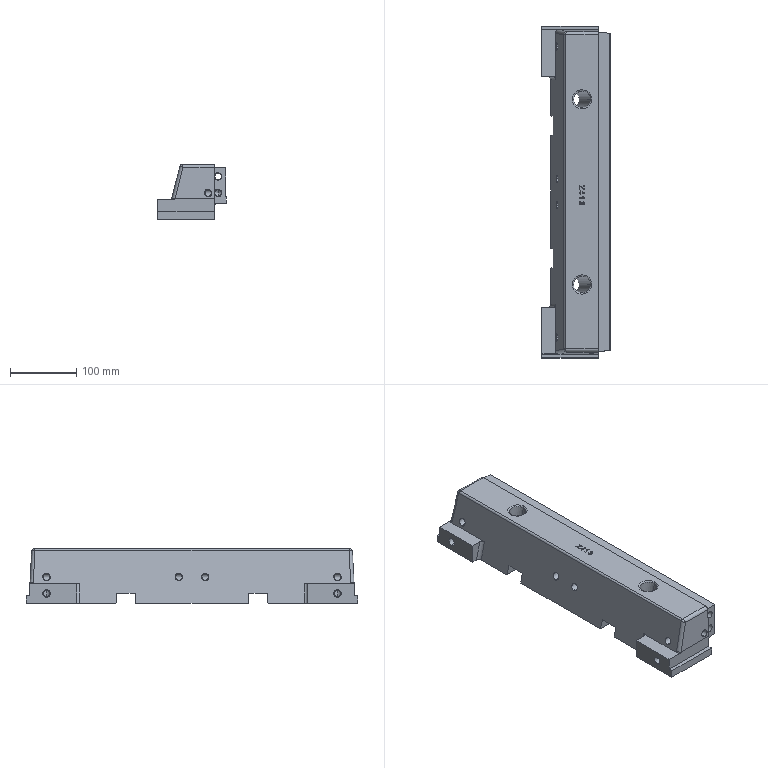Part | Creo | 1 solid | 213 faces | box 103.035 x 502 x 83 mm | volume 2737070 mm3 | cylinder 103 | plane 92 | spline 8 | other 6 | cone 4 | commonest cylinder face diameters 10 x52 11.4 x32 16 x6 12 x4 25 x4 2 x2